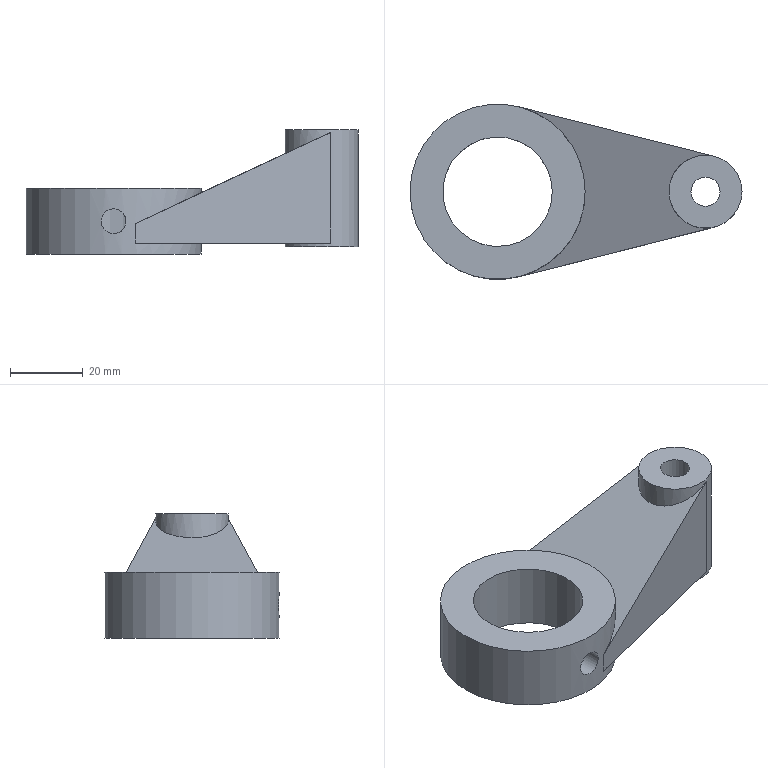Part | NX | features EXTRUDE 6, DATUM_CSYS 5, SKETCH 4, REPLACE_FACE 3, BLEND 2, DATUM_PLANE 1, HOLE PACKAGE 1, SIMPLE HOLE 1, SYMBOLIC_THREAD 1, UNITE 1 | 1 solid | 31 faces | box 91 x 48 x 34 mm | volume 35524 mm3 | plane 13 | cylinder 12 | sphere 4 | spline 2 | commonest cylinder face diameters 4 x6 6.8 x1 8 x1 14.5 x1 20 x1 30 x1
STEP:
#1=CARTESIAN_POINT('',(-3.4,-23.758,9.));
#2=VERTEX_POINT('',#1);
#3=CARTESIAN_POINT('',(-2.662,-23.88,6.333));
#4=CARTESIAN_POINT('',(-3.769,-23.697,9.001));
#5=CARTESIAN_POINT('',(-2.663,-23.88,11.665));
#6=CARTESIAN_POINT('',(-0.003138,-24.06,12.767));
#7=CARTESIAN_POINT('',(2.664,-23.88,11.665));
#8=CARTESIAN_POINT('',(3.767,-23.697,9.001));
#9=CARTESIAN_POINT('',(2.667,-23.879,6.339));
#10=CARTESIAN_POINT('',(0.003174,-24.06,5.232));
#11=CARTESIAN_POINT('',(-2.662,-23.88,6.333));
#12=CARTESIAN_POINT('',(-3.769,-23.697,9.001));
#13=CARTESIAN_POINT('',(-2.663,-23.88,11.665));
#14=B_SPLINE_CURVE_WITH_KNOTS('',3,(#3,#4,#5,#6,#7,#8,#9,#10,#11,#12,#13),.UNSPECIFIED.,.T.,.F.,(1,1,1,1,1,1,1,1,1,1,1,1,1,1,1),(-0.007982,-0.005321,-0.002661,0.,0.002661,0.005321,0.007982,0.01064,0.0133,0.01596,0.01862,0.02128,0.02394,0.02661,0.02927),.UNSPECIFIED.);
#15=EDGE_CURVE('',#2,#2,#14,.T.);
#16=ORIENTED_EDGE('',*,*,#15,.T.);
#17=EDGE_LOOP('',(#16));
#18=FACE_BOUND('',#17,.T.);
#19=CARTESIAN_POINT('',(5.895,23.265,3.));
#20=VERTEX_POINT('',#19);
#21=CARTESIAN_POINT('',(21.457,10.751,3.));
#22=VERTEX_POINT('',#21);
#23=CARTESIAN_POINT('',(0.,0.,3.));
#24=DIRECTION('',(0.,0.,-1.));
#25=DIRECTION('',(1.,0.,0.));
#26=AXIS2_PLACEMENT_3D('',#23,#24,#25);
#27=CIRCLE('',#26,24.);
#28=EDGE_CURVE('',#20,#22,#27,.T.);
#29=ORIENTED_EDGE('',*,*,#28,.T.);
#30=CARTESIAN_POINT('',(21.457,10.751,8.699));
#31=VERTEX_POINT('',#30);
#32=CARTESIAN_POINT('',(21.457,10.751,18.));
#33=DIRECTION('',(0.,0.,-1.));
#34=VECTOR('',#33,1000.);
#35=LINE('',#32,#34);
#36=EDGE_CURVE('',#22,#31,#35,.F.);
#37=ORIENTED_EDGE('',*,*,#36,.T.);
#38=CARTESIAN_POINT('',(21.457,-10.751,8.699));
#39=VERTEX_POINT('',#38);
#40=CARTESIAN_POINT('',(0.,0.,-2.14));
#41=DIRECTION('',(-0.4509,0.,0.8926));
#42=DIRECTION('',(-0.8926,0.,-0.4509));
#43=AXIS2_PLACEMENT_3D('',#40,#41,#42);
#44=ELLIPSE('',#43,26.888,24.);
#45=EDGE_CURVE('',#31,#39,#44,.F.);
#46=ORIENTED_EDGE('',*,*,#45,.T.);
#47=CARTESIAN_POINT('',(21.457,-10.751,3.));
#48=VERTEX_POINT('',#47);
#49=CARTESIAN_POINT('',(21.457,-10.751,18.));
#50=DIRECTION('',(0.,0.,-1.));
#51=VECTOR('',#50,1000.);
#52=LINE('',#49,#51);
#53=EDGE_CURVE('',#39,#48,#52,.T.);
#54=ORIENTED_EDGE('',*,*,#53,.T.);
#55=CARTESIAN_POINT('',(5.895,-23.265,3.));
#56=VERTEX_POINT('',#55);
#57=CARTESIAN_POINT('',(0.,0.,3.));
#58=DIRECTION('',(0.,0.,-1.));
#59=DIRECTION('',(1.,0.,0.));
#60=AXIS2_PLACEMENT_3D('',#57,#58,#59);
#61=CIRCLE('',#60,24.);
#62=EDGE_CURVE('',#48,#56,#61,.T.);
#63=ORIENTED_EDGE('',*,*,#62,.T.);
#64=CARTESIAN_POINT('',(5.895,-23.265,8.332));
#65=VERTEX_POINT('',#64);
#66=CARTESIAN_POINT('',(5.895,-23.265,43.));
#67=DIRECTION('',(0.,0.,-1.));
#68=VECTOR('',#67,1000.);
#69=LINE('',#66,#68);
#70=EDGE_CURVE('',#65,#56,#69,.T.);
#71=ORIENTED_EDGE('',*,*,#70,.F.);
#72=CARTESIAN_POINT('',(5.895,23.265,8.332));
#73=VERTEX_POINT('',#72);
#74=CARTESIAN_POINT('',(0.,0.,5.584));
#75=DIRECTION('',(-0.4226,0.,0.9063));
#76=DIRECTION('',(0.9063,0.,0.4226));
#77=AXIS2_PLACEMENT_3D('',#74,#75,#76);
#78=ELLIPSE('',#77,26.481,24.);
#79=EDGE_CURVE('',#73,#65,#78,.F.);
#80=ORIENTED_EDGE('',*,*,#79,.F.);
#81=CARTESIAN_POINT('',(5.895,23.265,43.));
#82=DIRECTION('',(0.,0.,-1.));
#83=VECTOR('',#82,1000.);
#84=LINE('',#81,#83);
#85=EDGE_CURVE('',#73,#20,#84,.T.);
#86=ORIENTED_EDGE('',*,*,#85,.T.);
#87=EDGE_LOOP('',(#29,#37,#46,#54,#63,#71,#80,#86));
#88=FACE_BOUND('',#87,.T.);
#89=CARTESIAN_POINT('',(24.,0.,0.));
#90=VERTEX_POINT('',#89);
#91=CARTESIAN_POINT('',(0.,0.,0.));
#92=DIRECTION('',(0.,0.,1.));
#93=DIRECTION('',(1.,0.,0.));
#94=AXIS2_PLACEMENT_3D('',#91,#92,#93);
#95=CIRCLE('',#94,24.);
#96=EDGE_CURVE('',#90,#90,#95,.T.);
#97=ORIENTED_EDGE('',*,*,#96,.T.);
#98=EDGE_LOOP('',(#97));
#99=FACE_BOUND('',#98,.T.);
#100=CARTESIAN_POINT('',(24.,0.,18.));
#101=VERTEX_POINT('',#100);
#102=CARTESIAN_POINT('',(0.,0.,18.));
#103=DIRECTION('',(0.,0.,1.));
#104=DIRECTION('',(1.,0.,0.));
#105=AXIS2_PLACEMENT_3D('',#102,#103,#104);
#106=CIRCLE('',#105,24.);
#107=EDGE_CURVE('',#101,#101,#106,.T.);
#108=ORIENTED_EDGE('',*,*,#107,.F.);
#109=EDGE_LOOP('',(#108));
#110=FACE_BOUND('',#109,.T.);
#111=CARTESIAN_POINT('',(0.,0.,18.));
#112=DIRECTION('',(0.,0.,-1.));
#113=DIRECTION('',(-1.,0.,0.));
#114=AXIS2_PLACEMENT_3D('',#111,#112,#113);
#115=CYLINDRICAL_SURFACE('',#114,24.);
#116=ADVANCED_FACE('',(#18,#88,#99,#110),#115,.T.);
#117=CARTESIAN_POINT('',(-3.4,-14.61,9.));
#118=VERTEX_POINT('',#117);
#119=CARTESIAN_POINT('',(-2.662,-14.808,6.333));
#120=CARTESIAN_POINT('',(-3.769,-14.511,9.001));
#121=CARTESIAN_POINT('',(-2.663,-14.807,11.665));
#122=CARTESIAN_POINT('',(-0.00369,-15.096,12.768));
#123=CARTESIAN_POINT('',(2.665,-14.807,11.664));
#124=CARTESIAN_POINT('',(3.767,-14.511,9.001));
#125=CARTESIAN_POINT('',(2.667,-14.807,6.338));
#126=CARTESIAN_POINT('',(0.001855,-15.096,5.232));
#127=CARTESIAN_POINT('',(-2.662,-14.808,6.333));
#128=CARTESIAN_POINT('',(-3.769,-14.511,9.001));
#129=CARTESIAN_POINT('',(-2.663,-14.807,11.665));
#130=B_SPLINE_CURVE_WITH_KNOTS('',3,(#119,#120,#121,#122,#123,#124,#125,#126,#127,#128,#129),.UNSPECIFIED.,.T.,.F.,(1,1,1,1,1,1,1,1,1,1,1,1,1,1,1),(-0.007997,-0.005332,-0.002666,0.,0.002666,0.005332,0.007997,0.01066,0.01333,0.01599,0.01866,0.02133,0.02399,0.02666,0.02932),.UNSPECIFIED.);
#131=EDGE_CURVE('',#118,#118,#130,.T.);
#132=ORIENTED_EDGE('',*,*,#131,.F.);
#133=EDGE_LOOP('',(#132));
#134=FACE_BOUND('',#133,.T.);
#135=CARTESIAN_POINT('',(15.,0.,18.));
#136=VERTEX_POINT('',#135);
#137=CARTESIAN_POINT('',(0.,0.,18.));
#138=DIRECTION('',(0.,0.,1.));
#139=DIRECTION('',(1.,0.,0.));
#140=AXIS2_PLACEMENT_3D('',#137,#138,#139);
#141=CIRCLE('',#140,15.);
#142=EDGE_CURVE('',#136,#136,#141,.T.);
#143=ORIENTED_EDGE('',*,*,#142,.T.);
#144=EDGE_LOOP('',(#143));
#145=FACE_BOUND('',#144,.T.);
#146=CARTESIAN_POINT('',(15.,0.,0.));
#147=VERTEX_POINT('',#146);
#148=CARTESIAN_POINT('',(0.,0.,0.));
#149=DIRECTION('',(0.,0.,1.));
#150=DIRECTION('',(1.,0.,0.));
#151=AXIS2_PLACEMENT_3D('',#148,#149,#150);
#152=CIRCLE('',#151,15.);
#153=EDGE_CURVE('',#147,#147,#152,.T.);
#154=ORIENTED_EDGE('',*,*,#153,.F.);
#155=EDGE_LOOP('',(#154));
#156=FACE_BOUND('',#155,.T.);
#157=CARTESIAN_POINT('',(0.,0.,18.));
#158=DIRECTION('',(0.,0.,-1.));
#159=DIRECTION('',(-1.,0.,0.));
#160=AXIS2_PLACEMENT_3D('',#157,#158,#159);
#161=CYLINDRICAL_SURFACE('',#160,15.);
#162=ADVANCED_FACE('',(#134,#145,#156),#161,.F.);
#163=ORIENTED_EDGE('',*,*,#107,.T.);
#164=EDGE_LOOP('',(#163));
#165=FACE_BOUND('',#164,.T.);
#166=ORIENTED_EDGE('',*,*,#142,.F.);
#167=EDGE_LOOP('',(#166));
#168=FACE_BOUND('',#167,.T.);
#169=CARTESIAN_POINT('',(0.,0.,18.));
#170=DIRECTION('',(0.,0.,1.));
#171=DIRECTION('',(1.,0.,0.));
#172=AXIS2_PLACEMENT_3D('',#169,#170,#171);
#173=PLANE('',#172);
#174=ADVANCED_FACE('',(#165,#168),#173,.T.);
#175=ORIENTED_EDGE('',*,*,#96,.F.);
#176=EDGE_LOOP('',(#175));
#177=FACE_BOUND('',#176,.T.);
#178=ORIENTED_EDGE('',*,*,#153,.T.);
#179=EDGE_LOOP('',(#178));
#180=FACE_BOUND('',#179,.T.);
#181=CARTESIAN_POINT('',(0.,0.,0.));
#182=DIRECTION('',(0.,0.,1.));
#183=DIRECTION('',(1.,0.,0.));
#184=AXIS2_PLACEMENT_3D('',#181,#182,#183);
#185=PLANE('',#184);
#186=ADVANCED_FACE('',(#177,#180),#185,.F.);
#187=CARTESIAN_POINT('',(61.,0.,34.));
#188=VERTEX_POINT('',#187);
#189=CARTESIAN_POINT('',(57.,0.,34.));
#190=DIRECTION('',(0.,0.,1.));
#191=DIRECTION('',(1.,0.,0.));
#192=AXIS2_PLACEMENT_3D('',#189,#190,#191);
#193=CIRCLE('',#192,4.);
#194=EDGE_CURVE('',#188,#188,#193,.T.);
#195=ORIENTED_EDGE('',*,*,#194,.T.);
#196=EDGE_LOOP('',(#195));
#197=FACE_BOUND('',#196,.T.);
#198=CARTESIAN_POINT('',(53.,0.,27.));
#199=VERTEX_POINT('',#198);
#200=CARTESIAN_POINT('',(57.,0.,27.));
#201=DIRECTION('',(0.,0.,-1.));
#202=DIRECTION('',(-1.,0.,0.));
#203=AXIS2_PLACEMENT_3D('',#200,#201,#202);
#204=CIRCLE('',#203,4.);
#205=EDGE_CURVE('',#199,#199,#204,.T.);
#206=ORIENTED_EDGE('',*,*,#205,.T.);
#207=EDGE_LOOP('',(#206));
#208=FACE_BOUND('',#207,.T.);
#209=CARTESIAN_POINT('',(57.,0.,34.));
#210=DIRECTION('',(0.,0.,-1.));
#211=DIRECTION('',(-1.,0.,0.));
#212=AXIS2_PLACEMENT_3D('',#209,#210,#211);
#213=CYLINDRICAL_SURFACE('',#212,4.);
#214=ADVANCED_FACE('',(#197,#208),#213,.F.);
#215=CARTESIAN_POINT('',(48.228,4.802,19.531));
#216=VERTEX_POINT('',#215);
#217=CARTESIAN_POINT('',(48.228,4.802,3.));
#218=VERTEX_POINT('',#217);
#219=CARTESIAN_POINT('',(48.228,4.802,34.));
#220=DIRECTION('',(0.,0.,-1.));
#221=VECTOR('',#220,1000.);
#222=LINE('',#219,#221);
#223=EDGE_CURVE('',#216,#218,#222,.T.);
#224=ORIENTED_EDGE('',*,*,#223,.T.);
#225=CARTESIAN_POINT('',(59.456,9.694,3.));
#226=VERTEX_POINT('',#225);
#227=CARTESIAN_POINT('',(57.,0.,3.));
#228=DIRECTION('',(0.,0.,-1.));
#229=DIRECTION('',(1.,0.,0.));
#230=AXIS2_PLACEMENT_3D('',#227,#228,#229);
#231=CIRCLE('',#230,10.);
#232=EDGE_CURVE('',#218,#226,#231,.T.);
#233=ORIENTED_EDGE('',*,*,#232,.T.);
#234=CARTESIAN_POINT('',(59.456,9.694,33.308));
#235=VERTEX_POINT('',#234);
#236=CARTESIAN_POINT('',(59.456,9.694,30.55));
#237=DIRECTION('',(0.,0.,-1.));
#238=VECTOR('',#237,1000.);
#239=LINE('',#236,#238);
#240=EDGE_CURVE('',#226,#235,#239,.F.);
#241=ORIENTED_EDGE('',*,*,#240,.T.);
#242=CARTESIAN_POINT('',(59.456,-9.694,33.308));
#243=VERTEX_POINT('',#242);
#244=CARTESIAN_POINT('',(57.,0.,32.163));
#245=DIRECTION('',(-0.4226,0.,0.9063));
#246=DIRECTION('',(-0.9063,0.,-0.4226));
#247=AXIS2_PLACEMENT_3D('',#244,#245,#246);
#248=ELLIPSE('',#247,11.034,10.);
#249=EDGE_CURVE('',#235,#243,#248,.T.);
#250=ORIENTED_EDGE('',*,*,#249,.T.);
#251=CARTESIAN_POINT('',(59.456,-9.694,3.));
#252=VERTEX_POINT('',#251);
#253=CARTESIAN_POINT('',(59.456,-9.694,30.55));
#254=DIRECTION('',(0.,0.,-1.));
#255=VECTOR('',#254,1000.);
#256=LINE('',#253,#255);
#257=EDGE_CURVE('',#243,#252,#256,.T.);
#258=ORIENTED_EDGE('',*,*,#257,.T.);
#259=CARTESIAN_POINT('',(48.228,-4.802,3.));
#260=VERTEX_POINT('',#259);
#261=CARTESIAN_POINT('',(57.,0.,3.));
#262=DIRECTION('',(0.,0.,-1.));
#263=DIRECTION('',(1.,0.,0.));
#264=AXIS2_PLACEMENT_3D('',#261,#262,#263);
#265=CIRCLE('',#264,10.);
#266=EDGE_CURVE('',#252,#260,#265,.T.);
#267=ORIENTED_EDGE('',*,*,#266,.T.);
#268=CARTESIAN_POINT('',(48.228,-4.802,19.531));
#269=VERTEX_POINT('',#268);
#270=CARTESIAN_POINT('',(48.228,-4.802,34.));
#271=DIRECTION('',(0.,0.,-1.));
#272=VECTOR('',#271,1000.);
#273=LINE('',#270,#272);
#274=EDGE_CURVE('',#260,#269,#273,.F.);
#275=ORIENTED_EDGE('',*,*,#274,.T.);
#276=CARTESIAN_POINT('',(57.,0.,24.439));
#277=DIRECTION('',(-0.4883,0.,0.8727));
#278=DIRECTION('',(-0.8727,0.,-0.4883));
#279=AXIS2_PLACEMENT_3D('',#276,#277,#278);
#280=ELLIPSE('',#279,11.459,10.);
#281=EDGE_CURVE('',#269,#216,#280,.F.);
#282=ORIENTED_EDGE('',*,*,#281,.T.);
#283=EDGE_LOOP('',(#224,#233,#241,#250,#258,#267,#275,#282));
#284=FACE_BOUND('',#283,.T.);
#285=CARTESIAN_POINT('',(67.,0.,2.));
#286=VERTEX_POINT('',#285);
#287=CARTESIAN_POINT('',(57.,0.,2.));
#288=DIRECTION('',(0.,0.,1.));
#289=DIRECTION('',(1.,0.,0.));
#290=AXIS2_PLACEMENT_3D('',#287,#288,#289);
#291=CIRCLE('',#290,10.);
#292=EDGE_CURVE('',#286,#286,#291,.T.);
#293=ORIENTED_EDGE('',*,*,#292,.T.);
#294=EDGE_LOOP('',(#293));
#295=FACE_BOUND('',#294,.T.);
#296=CARTESIAN_POINT('',(67.,0.,34.));
#297=VERTEX_POINT('',#296);
#298=CARTESIAN_POINT('',(57.,0.,34.));
#299=DIRECTION('',(0.,0.,1.));
#300=DIRECTION('',(1.,0.,0.));
#301=AXIS2_PLACEMENT_3D('',#298,#299,#300);
#302=CIRCLE('',#301,10.);
#303=EDGE_CURVE('',#297,#297,#302,.T.);
#304=ORIENTED_EDGE('',*,*,#303,.F.);
#305=EDGE_LOOP('',(#304));
#306=FACE_BOUND('',#305,.T.);
#307=CARTESIAN_POINT('',(57.,0.,34.));
#308=DIRECTION('',(0.,0.,-1.));
#309=DIRECTION('',(-1.,0.,0.));
#310=AXIS2_PLACEMENT_3D('',#307,#308,#309);
#311=CYLINDRICAL_SURFACE('',#310,10.);
#312=ADVANCED_FACE('',(#284,#295,#306),#311,.T.);
#313=ORIENTED_EDGE('',*,*,#303,.T.);
#314=EDGE_LOOP('',(#313));
#315=FACE_BOUND('',#314,.T.);
#316=ORIENTED_EDGE('',*,*,#194,.F.);
#317=EDGE_LOOP('',(#316));
#318=FACE_BOUND('',#317,.T.);
#319=CARTESIAN_POINT('',(57.,0.,34.));
#320=DIRECTION('',(0.,0.,1.));
#321=DIRECTION('',(1.,0.,0.));
#322=AXIS2_PLACEMENT_3D('',#319,#320,#321);
#323=PLANE('',#322);
#324=ADVANCED_FACE('',(#315,#318),#323,.T.);
#325=CARTESIAN_POINT('',(64.25,0.,2.));
#326=VERTEX_POINT('',#325);
#327=CARTESIAN_POINT('',(57.,0.,2.));
#328=DIRECTION('',(0.,0.,-1.));
#329=DIRECTION('',(1.,0.,0.));
#330=AXIS2_PLACEMENT_3D('',#327,#328,#329);
#331=CIRCLE('',#330,7.25);
#332=EDGE_CURVE('',#326,#326,#331,.T.);
#333=ORIENTED_EDGE('',*,*,#332,.F.);
#334=EDGE_LOOP('',(#333));
#335=FACE_BOUND('',#334,.T.);
#336=ORIENTED_EDGE('',*,*,#292,.F.);
#337=EDGE_LOOP('',(#336));
#338=FACE_BOUND('',#337,.T.);
#339=CARTESIAN_POINT('',(57.,0.,2.));
#340=DIRECTION('',(0.,0.,1.));
#341=DIRECTION('',(1.,0.,0.));
#342=AXIS2_PLACEMENT_3D('',#339,#340,#341);
#343=PLANE('',#342);
#344=ADVANCED_FACE('',(#335,#338),#343,.F.);
#345=CARTESIAN_POINT('',(64.25,0.,27.));
#346=VERTEX_POINT('',#345);
#347=CARTESIAN_POINT('',(57.,0.,27.));
#348=DIRECTION('',(0.,0.,-1.));
#349=DIRECTION('',(1.,0.,0.));
#350=AXIS2_PLACEMENT_3D('',#347,#348,#349);
#351=CIRCLE('',#350,7.25);
#352=EDGE_CURVE('',#346,#346,#351,.F.);
#353=ORIENTED_EDGE('',*,*,#352,.T.);
#354=EDGE_LOOP('',(#353));
#355=FACE_BOUND('',#354,.T.);
#356=ORIENTED_EDGE('',*,*,#332,.T.);
#357=EDGE_LOOP('',(#356));
#358=FACE_BOUND('',#357,.T.);
#359=CARTESIAN_POINT('',(57.,0.,27.));
#360=DIRECTION('',(0.,0.,-1.));
#361=DIRECTION('',(-1.,0.,0.));
#362=AXIS2_PLACEMENT_3D('',#359,#360,#361);
#363=CYLINDRICAL_SURFACE('',#362,7.25);
#364=ADVANCED_FACE('',(#355,#358),#363,.F.);
#365=ORIENTED_EDGE('',*,*,#205,.F.);
#366=EDGE_LOOP('',(#365));
#367=FACE_BOUND('',#366,.T.);
#368=ORIENTED_EDGE('',*,*,#352,.F.);
#369=EDGE_LOOP('',(#368));
#370=FACE_BOUND('',#369,.T.);
#371=CARTESIAN_POINT('',(57.,0.,27.));
#372=DIRECTION('',(0.,0.,-1.));
#373=DIRECTION('',(-1.,0.,0.));
#374=AXIS2_PLACEMENT_3D('',#371,#372,#373);
#375=PLANE('',#374);
#376=ADVANCED_FACE('',(#367,#370),#375,.T.);
#377=CARTESIAN_POINT('',(46.965,-7.701,3.));
#378=VERTEX_POINT('',#377);
#379=CARTESIAN_POINT('',(23.736,-13.586,3.));
#380=VERTEX_POINT('',#379);
#381=CARTESIAN_POINT('',(49.833,-6.974,3.));
#382=DIRECTION('',(-0.9694,-0.2456,0.));
#383=VECTOR('',#382,1000.);
#384=LINE('',#381,#383);
#385=EDGE_CURVE('',#378,#380,#384,.T.);
#386=ORIENTED_EDGE('',*,*,#385,.T.);
#387=CARTESIAN_POINT('',(23.736,-13.586,8.699));
#388=VERTEX_POINT('',#387);
#389=CARTESIAN_POINT('',(23.736,-13.586,6.435));
#390=DIRECTION('',(0.,0.,1.));
#391=VECTOR('',#390,1000.);
#392=LINE('',#389,#391);
#393=EDGE_CURVE('',#380,#388,#392,.T.);
#394=ORIENTED_EDGE('',*,*,#393,.T.);
#395=CARTESIAN_POINT('',(46.965,-7.701,19.531));
#396=VERTEX_POINT('',#395);
#397=CARTESIAN_POINT('',(57.885,-4.934,24.623));
#398=DIRECTION('',(-0.8833,-0.2238,-0.4119));
#399=VECTOR('',#398,1000.);
#400=LINE('',#397,#399);
#401=EDGE_CURVE('',#388,#396,#400,.F.);
#402=ORIENTED_EDGE('',*,*,#401,.T.);
#403=CARTESIAN_POINT('',(46.965,-7.701,3.));
#404=DIRECTION('',(0.,0.,1.));
#405=VECTOR('',#404,1000.);
#406=LINE('',#403,#405);
#407=EDGE_CURVE('',#396,#378,#406,.F.);
#408=ORIENTED_EDGE('',*,*,#407,.T.);
#409=EDGE_LOOP('',(#386,#394,#402,#408));
#410=FACE_BOUND('',#409,.T.);
#411=CARTESIAN_POINT('',(49.833,-6.974,43.));
#412=DIRECTION('',(0.2456,-0.9694,0.));
#413=DIRECTION('',(0.9694,0.2456,0.));
#414=AXIS2_PLACEMENT_3D('',#411,#412,#413);
#415=PLANE('',#414);
#416=ADVANCED_FACE('',(#410),#415,.F.);
#417=ORIENTED_EDGE('',*,*,#62,.F.);
#418=CARTESIAN_POINT('',(23.245,-11.647,3.));
#419=DIRECTION('',(0.,0.,-1.));
#420=DIRECTION('',(-1.,0.,0.));
#421=AXIS2_PLACEMENT_3D('',#418,#419,#420);
#422=CIRCLE('',#421,2.);
#423=EDGE_CURVE('',#48,#380,#422,.F.);
#424=ORIENTED_EDGE('',*,*,#423,.T.);
#425=ORIENTED_EDGE('',*,*,#385,.F.);
#426=CARTESIAN_POINT('',(46.474,-5.762,3.));
#427=DIRECTION('',(0.,0.,-1.));
#428=DIRECTION('',(-1.,0.,0.));
#429=AXIS2_PLACEMENT_3D('',#426,#427,#428);
#430=CIRCLE('',#429,2.);
#431=EDGE_CURVE('',#378,#260,#430,.F.);
#432=ORIENTED_EDGE('',*,*,#431,.T.);
#433=ORIENTED_EDGE('',*,*,#266,.F.);
#434=CARTESIAN_POINT('',(5.895,-23.265,3.));
#435=DIRECTION('',(0.9694,0.2456,0.));
#436=VECTOR('',#435,1000.);
#437=LINE('',#434,#436);
#438=EDGE_CURVE('',#56,#252,#437,.T.);
#439=ORIENTED_EDGE('',*,*,#438,.F.);
#440=EDGE_LOOP('',(#417,#424,#425,#432,#433,#439));
#441=FACE_BOUND('',#440,.T.);
#442=CARTESIAN_POINT('',(0.,0.,3.));
#443=DIRECTION('',(0.,0.,-1.));
#444=DIRECTION('',(-1.,0.,0.));
#445=AXIS2_PLACEMENT_3D('',#442,#443,#444);
#446=PLANE('',#445);
#447=ADVANCED_FACE('',(#441),#446,.T.);
#448=CARTESIAN_POINT('',(46.965,7.701,19.531));
#449=VERTEX_POINT('',#448);
#450=CARTESIAN_POINT('',(23.736,13.586,8.699));
#451=VERTEX_POINT('',#450);
#452=CARTESIAN_POINT('',(32.184,11.446,12.639));
#453=DIRECTION('',(0.8833,-0.2238,0.4119));
#454=VECTOR('',#453,1000.);
#455=LINE('',#452,#454);
#456=EDGE_CURVE('',#449,#451,#455,.F.);
#457=ORIENTED_EDGE('',*,*,#456,.T.);
#458=CARTESIAN_POINT('',(23.736,13.586,3.));
#459=VERTEX_POINT('',#458);
#460=CARTESIAN_POINT('',(23.736,13.586,3.));
#461=DIRECTION('',(0.,0.,1.));
#462=VECTOR('',#461,1000.);
#463=LINE('',#460,#462);
#464=EDGE_CURVE('',#451,#459,#463,.F.);
#465=ORIENTED_EDGE('',*,*,#464,.T.);
#466=CARTESIAN_POINT('',(46.965,7.701,3.));
#467=VERTEX_POINT('',#466);
#468=CARTESIAN_POINT('',(18.88,14.817,3.));
#469=DIRECTION('',(0.9694,-0.2456,0.));
#470=VECTOR('',#469,1000.);
#471=LINE('',#468,#470);
#472=EDGE_CURVE('',#459,#467,#471,.T.);
#473=ORIENTED_EDGE('',*,*,#472,.T.);
#474=CARTESIAN_POINT('',(46.965,7.701,23.304));
#475=DIRECTION('',(0.,0.,1.));
#476=VECTOR('',#475,1000.);
#477=LINE('',#474,#476);
#478=EDGE_CURVE('',#467,#449,#477,.T.);
#479=ORIENTED_EDGE('',*,*,#478,.T.);
#480=EDGE_LOOP('',(#457,#465,#473,#479));
#481=FACE_BOUND('',#480,.T.);
#482=CARTESIAN_POINT('',(18.88,14.817,43.));
#483=DIRECTION('',(0.2456,0.9694,0.));
#484=DIRECTION('',(-0.9694,0.2456,0.));
#485=AXIS2_PLACEMENT_3D('',#482,#483,#484);
#486=PLANE('',#485);
#487=ADVANCED_FACE('',(#481),#486,.F.);
#488=ORIENTED_EDGE('',*,*,#28,.F.);
#489=CARTESIAN_POINT('',(59.456,9.694,3.));
#490=DIRECTION('',(-0.9694,0.2456,0.));
#491=VECTOR('',#490,1000.);
#492=LINE('',#489,#491);
#493=EDGE_CURVE('',#226,#20,#492,.T.);
#494=ORIENTED_EDGE('',*,*,#493,.F.);
#495=ORIENTED_EDGE('',*,*,#232,.F.);
#496=CARTESIAN_POINT('',(46.474,5.762,3.));
#497=DIRECTION('',(0.,0.,-1.));
#498=DIRECTION('',(-1.,0.,0.));
#499=AXIS2_PLACEMENT_3D('',#496,#497,#498);
#500=CIRCLE('',#499,2.);
#501=EDGE_CURVE('',#218,#467,#500,.F.);
#502=ORIENTED_EDGE('',*,*,#501,.T.);
#503=ORIENTED_EDGE('',*,*,#472,.F.);
#504=CARTESIAN_POINT('',(23.245,11.647,3.));
#505=DIRECTION('',(0.,0.,-1.));
#506=DIRECTION('',(-1.,0.,0.));
#507=AXIS2_PLACEMENT_3D('',#504,#505,#506);
#508=CIRCLE('',#507,2.);
#509=EDGE_CURVE('',#459,#22,#508,.F.);
#510=ORIENTED_EDGE('',*,*,#509,.T.);
#511=EDGE_LOOP('',(#488,#494,#495,#502,#503,#510));
#512=FACE_BOUND('',#511,.T.);
#513=CARTESIAN_POINT('',(0.,0.,3.));
#514=DIRECTION('',(0.,0.,-1.));
#515=DIRECTION('',(-1.,0.,0.));
#516=AXIS2_PLACEMENT_3D('',#513,#514,#515);
#517=PLANE('',#516);
#518=ADVANCED_FACE('',(#512),#517,.T.);
#519=ORIENTED_EDGE('',*,*,#85,.F.);
#520=CARTESIAN_POINT('',(44.598,13.458,26.38));
#521=DIRECTION('',(-0.8833,0.2238,-0.4119));
#522=VECTOR('',#521,1000.);
#523=LINE('',#520,#522);
#524=EDGE_CURVE('',#235,#73,#523,.T.);
#525=ORIENTED_EDGE('',*,*,#524,.F.);
#526=ORIENTED_EDGE('',*,*,#240,.F.);
#527=ORIENTED_EDGE('',*,*,#493,.T.);
#528=EDGE_LOOP('',(#519,#525,#526,#527));
#529=FACE_BOUND('',#528,.T.);
#530=CARTESIAN_POINT('',(59.456,9.694,-25.));
#531=DIRECTION('',(0.2456,0.9694,0.));
#532=DIRECTION('',(-0.9694,0.2456,0.));
#533=AXIS2_PLACEMENT_3D('',#530,#531,#532);
#534=PLANE('',#533);
#535=ADVANCED_FACE('',(#529),#534,.T.);
#536=CARTESIAN_POINT('',(54.483,-10.954,30.989));
#537=DIRECTION('',(0.8833,0.2238,0.4119));
#538=VECTOR('',#537,1000.);
#539=LINE('',#536,#538);
#540=EDGE_CURVE('',#65,#243,#539,.T.);
#541=ORIENTED_EDGE('',*,*,#540,.F.);
#542=ORIENTED_EDGE('',*,*,#70,.T.);
#543=ORIENTED_EDGE('',*,*,#438,.T.);
#544=ORIENTED_EDGE('',*,*,#257,.F.);
#545=EDGE_LOOP('',(#541,#542,#543,#544));
#546=FACE_BOUND('',#545,.T.);
#547=CARTESIAN_POINT('',(5.895,-23.265,-25.));
#548=DIRECTION('',(0.2456,-0.9694,0.));
#549=DIRECTION('',(0.9694,0.2456,0.));
#550=AXIS2_PLACEMENT_3D('',#547,#548,#549);
#551=PLANE('',#550);
#552=ADVANCED_FACE('',(#546),#551,.T.);
#553=ORIENTED_EDGE('',*,*,#79,.T.);
#554=ORIENTED_EDGE('',*,*,#540,.T.);
#555=ORIENTED_EDGE('',*,*,#249,.F.);
#556=ORIENTED_EDGE('',*,*,#524,.T.);
#557=EDGE_LOOP('',(#553,#554,#555,#556));
#558=FACE_BOUND('',#557,.T.);
#559=CARTESIAN_POINT('',(47.,25.,27.5));
#560=DIRECTION('',(-0.4226,0.,0.9063));
#561=DIRECTION('',(0.9063,0.,0.4226));
#562=AXIS2_PLACEMENT_3D('',#559,#560,#561);
#563=PLANE('',#562);
#564=ADVANCED_FACE('',(#558),#563,.T.);
#565=CARTESIAN_POINT('',(45.629,-5.762,21.344));
#566=VERTEX_POINT('',#565);
#567=CARTESIAN_POINT('',(22.4,-11.647,10.512));
#568=VERTEX_POINT('',#567);
#569=CARTESIAN_POINT('',(19.614,-12.353,9.213));
#570=DIRECTION('',(-0.8833,-0.2238,-0.4119));
#571=VECTOR('',#570,1000.);
#572=LINE('',#569,#571);
#573=EDGE_CURVE('',#566,#568,#572,.T.);
#574=ORIENTED_EDGE('',*,*,#573,.T.);
#575=CARTESIAN_POINT('',(22.4,11.647,10.512));
#576=VERTEX_POINT('',#575);
#577=CARTESIAN_POINT('',(-0.8452,0.,-0.3275));
#578=DIRECTION('',(0.4226,0.,-0.9063));
#579=DIRECTION('',(-0.9063,0.,-0.4226));
#580=AXIS2_PLACEMENT_3D('',#577,#578,#579);
#581=ELLIPSE('',#580,28.688,26.);
#582=EDGE_CURVE('',#568,#576,#581,.F.);
#583=ORIENTED_EDGE('',*,*,#582,.T.);
#584=CARTESIAN_POINT('',(45.629,5.762,21.344));
#585=VERTEX_POINT('',#584);
#586=CARTESIAN_POINT('',(9.729,14.858,4.603));
#587=DIRECTION('',(0.8833,-0.2238,0.4119));
#588=VECTOR('',#587,1000.);
#589=LINE('',#586,#588);
#590=EDGE_CURVE('',#576,#585,#589,.T.);
#591=ORIENTED_EDGE('',*,*,#590,.T.);
#592=CARTESIAN_POINT('',(56.155,0.,26.252));
#593=DIRECTION('',(0.4226,0.,-0.9063));
#594=DIRECTION('',(-0.9063,0.,-0.4226));
#595=AXIS2_PLACEMENT_3D('',#592,#593,#594);
#596=ELLIPSE('',#595,13.241,12.);
#597=EDGE_CURVE('',#585,#566,#596,.F.);
#598=ORIENTED_EDGE('',*,*,#597,.T.);
#599=EDGE_LOOP('',(#574,#583,#591,#598));
#600=FACE_BOUND('',#599,.T.);
#601=CARTESIAN_POINT('',(11.84,25.,5.588));
#602=DIRECTION('',(0.4226,0.,-0.9063));
#603=DIRECTION('',(-0.9063,0.,-0.4226));
#604=AXIS2_PLACEMENT_3D('',#601,#602,#603);
#605=PLANE('',#604);
#606=ADVANCED_FACE('',(#600),#605,.T.);
#607=ORIENTED_EDGE('',*,*,#401,.F.);
#608=CARTESIAN_POINT('',(23.245,-11.647,8.699));
#609=DIRECTION('',(-0.8833,-0.2238,-0.4119));
#610=DIRECTION('',(-0.4226,0.,0.9063));
#611=AXIS2_PLACEMENT_3D('',#608,#609,#610);
#612=CIRCLE('',#611,2.);
#613=EDGE_CURVE('',#388,#568,#612,.T.);
#614=ORIENTED_EDGE('',*,*,#613,.T.);
#615=ORIENTED_EDGE('',*,*,#573,.F.);
#616=CARTESIAN_POINT('',(46.474,-5.762,19.531));
#617=DIRECTION('',(-0.8833,-0.2238,-0.4119));
#618=DIRECTION('',(-0.4226,0.,0.9063));
#619=AXIS2_PLACEMENT_3D('',#616,#617,#618);
#620=CIRCLE('',#619,2.);
#621=EDGE_CURVE('',#396,#566,#620,.T.);
#622=ORIENTED_EDGE('',*,*,#621,.F.);
#623=EDGE_LOOP('',(#607,#614,#615,#622));
#624=FACE_BOUND('',#623,.T.);
#625=CARTESIAN_POINT('',(20.459,-12.353,7.4));
#626=DIRECTION('',(-0.8833,-0.2238,-0.4119));
#627=DIRECTION('',(-0.4226,0.,0.9063));
#628=AXIS2_PLACEMENT_3D('',#625,#626,#627);
#629=CYLINDRICAL_SURFACE('',#628,2.);
#630=ADVANCED_FACE('',(#624),#629,.F.);
#631=ORIENTED_EDGE('',*,*,#431,.F.);
#632=ORIENTED_EDGE('',*,*,#407,.F.);
#633=CARTESIAN_POINT('',(46.474,-5.762,19.531));
#634=DIRECTION('',(0.,0.,-1.));
#635=DIRECTION('',(0.,1.,0.));
#636=AXIS2_PLACEMENT_3D('',#633,#634,#635);
#637=CIRCLE('',#636,2.);
#638=EDGE_CURVE('',#269,#396,#637,.T.);
#639=ORIENTED_EDGE('',*,*,#638,.F.);
#640=ORIENTED_EDGE('',*,*,#274,.F.);
#641=EDGE_LOOP('',(#631,#632,#639,#640));
#642=FACE_BOUND('',#641,.T.);
#643=CARTESIAN_POINT('',(46.474,-5.762,34.));
#644=DIRECTION('',(0.,0.,-1.));
#645=DIRECTION('',(-1.,0.,0.));
#646=AXIS2_PLACEMENT_3D('',#643,#644,#645);
#647=CYLINDRICAL_SURFACE('',#646,2.);
#648=ADVANCED_FACE('',(#642),#647,.F.);
#649=ORIENTED_EDGE('',*,*,#638,.T.);
#650=ORIENTED_EDGE('',*,*,#621,.T.);
#651=CARTESIAN_POINT('',(46.474,-5.762,19.531));
#652=DIRECTION('',(-0.4686,0.856,-0.2185));
#653=DIRECTION('',(-0.8772,-0.4802,0.));
#654=AXIS2_PLACEMENT_3D('',#651,#652,#653);
#655=CIRCLE('',#654,2.);
#656=EDGE_CURVE('',#269,#566,#655,.F.);
#657=ORIENTED_EDGE('',*,*,#656,.F.);
#658=EDGE_LOOP('',(#649,#650,#657));
#659=FACE_BOUND('',#658,.T.);
#660=CARTESIAN_POINT('',(46.474,-5.762,19.531));
#661=DIRECTION('',(0.,0.,1.));
#662=DIRECTION('',(1.,0.,0.));
#663=AXIS2_PLACEMENT_3D('',#660,#661,#662);
#664=SPHERICAL_SURFACE('',#663,2.);
#665=ADVANCED_FACE('',(#659),#664,.F.);
#666=ORIENTED_EDGE('',*,*,#656,.T.);
#667=ORIENTED_EDGE('',*,*,#597,.F.);
#668=CARTESIAN_POINT('',(46.474,5.762,19.531));
#669=DIRECTION('',(-0.4686,-0.856,-0.2185));
#670=DIRECTION('',(0.8772,-0.4802,0.));
#671=AXIS2_PLACEMENT_3D('',#668,#669,#670);
#672=CIRCLE('',#671,2.);
#673=EDGE_CURVE('',#216,#585,#672,.T.);
#674=ORIENTED_EDGE('',*,*,#673,.F.);
#675=ORIENTED_EDGE('',*,*,#281,.F.);
#676=EDGE_LOOP('',(#666,#667,#674,#675));
#677=FACE_BOUND('',#676,.T.);
#678=CARTESIAN_POINT('',(48.228,-4.802,19.531));
#679=CARTESIAN_POINT('',(47.919,-4.236,22.411));
#680=CARTESIAN_POINT('',(45.629,-5.762,21.344));
#681=CARTESIAN_POINT('',(47.427,-3.337,19.082));
#682=CARTESIAN_POINT('',(47.272,-2.824,22.11));
#683=CARTESIAN_POINT('',(44.667,-4.005,20.895));
#684=CARTESIAN_POINT('',(46.573,0.,18.605));
#685=CARTESIAN_POINT('',(46.72,0.,21.852));
#686=CARTESIAN_POINT('',(43.643,0.,20.418));
#687=CARTESIAN_POINT('',(47.427,3.337,19.082));
#688=CARTESIAN_POINT('',(47.272,2.824,22.11));
#689=CARTESIAN_POINT('',(44.667,4.005,20.895));
#690=CARTESIAN_POINT('',(48.228,4.802,19.531));
#691=CARTESIAN_POINT('',(47.919,4.236,22.411));
#692=CARTESIAN_POINT('',(45.629,5.762,21.344));
#693=(BOUNDED_SURFACE()B_SPLINE_SURFACE(3,2,((#678,#679,#680),(#681,#682,#683),(#684,#685,#686),(#687,#688,#689),(#690,#691,#692)),.UNSPECIFIED.,.F.,.F.,.F.)B_SPLINE_SURFACE_WITH_KNOTS((4,1,4),(3,3),(5.782,6.283,6.784),(0.,1.),.UNSPECIFIED.)GEOMETRIC_REPRESENTATION_ITEM()RATIONAL_B_SPLINE_SURFACE(((1.,0.5609,1.),(1.,0.5458,1.),(1.,0.5288,1.),(1.,0.5458,1.),(1.,0.5609,1.)))REPRESENTATION_ITEM('')SURFACE());
#694=ADVANCED_FACE('',(#677),#693,.F.);
#695=ORIENTED_EDGE('',*,*,#501,.F.);
#696=ORIENTED_EDGE('',*,*,#223,.F.);
#697=CARTESIAN_POINT('',(46.474,5.762,19.531));
#698=DIRECTION('',(0.,0.,-1.));
#699=DIRECTION('',(-1.,0.,0.));
#700=AXIS2_PLACEMENT_3D('',#697,#698,#699);
#701=CIRCLE('',#700,2.);
#702=EDGE_CURVE('',#449,#216,#701,.T.);
#703=ORIENTED_EDGE('',*,*,#702,.F.);
#704=ORIENTED_EDGE('',*,*,#478,.F.);
#705=EDGE_LOOP('',(#695,#696,#703,#704));
#706=FACE_BOUND('',#705,.T.);
#707=CARTESIAN_POINT('',(46.474,5.762,34.));
#708=DIRECTION('',(0.,0.,-1.));
#709=DIRECTION('',(-1.,0.,0.));
#710=AXIS2_PLACEMENT_3D('',#707,#708,#709);
#711=CYLINDRICAL_SURFACE('',#710,2.);
#712=ADVANCED_FACE('',(#706),#711,.F.);
#713=ORIENTED_EDGE('',*,*,#702,.T.);
#714=ORIENTED_EDGE('',*,*,#673,.T.);
#715=CARTESIAN_POINT('',(46.474,5.762,19.531));
#716=DIRECTION('',(-0.8833,0.2238,-0.4119));
#717=DIRECTION('',(-0.4226,0.,0.9063));
#718=AXIS2_PLACEMENT_3D('',#715,#716,#717);
#719=CIRCLE('',#718,2.);
#720=EDGE_CURVE('',#449,#585,#719,.F.);
#721=ORIENTED_EDGE('',*,*,#720,.F.);
#722=EDGE_LOOP('',(#713,#714,#721));
#723=FACE_BOUND('',#722,.T.);
#724=CARTESIAN_POINT('',(46.474,5.762,19.531));
#725=DIRECTION('',(0.,0.,1.));
#726=DIRECTION('',(1.,0.,0.));
#727=AXIS2_PLACEMENT_3D('',#724,#725,#726);
#728=SPHERICAL_SURFACE('',#727,2.);
#729=ADVANCED_FACE('',(#723),#728,.F.);
#730=ORIENTED_EDGE('',*,*,#590,.F.);
#731=CARTESIAN_POINT('',(23.245,11.647,8.699));
#732=DIRECTION('',(0.8833,-0.2238,0.4119));
#733=DIRECTION('',(0.4226,0.,-0.9063));
#734=AXIS2_PLACEMENT_3D('',#731,#732,#733);
#735=CIRCLE('',#734,2.);
#736=EDGE_CURVE('',#576,#451,#735,.F.);
#737=ORIENTED_EDGE('',*,*,#736,.T.);
#738=ORIENTED_EDGE('',*,*,#456,.F.);
#739=ORIENTED_EDGE('',*,*,#720,.T.);
#740=EDGE_LOOP('',(#730,#737,#738,#739));
#741=FACE_BOUND('',#740,.T.);
#742=CARTESIAN_POINT('',(10.574,14.858,2.791));
#743=DIRECTION('',(0.8833,-0.2238,0.4119));
#744=DIRECTION('',(0.4226,0.,-0.9063));
#745=AXIS2_PLACEMENT_3D('',#742,#743,#744);
#746=CYLINDRICAL_SURFACE('',#745,2.);
#747=ADVANCED_FACE('',(#741),#746,.F.);
#748=CARTESIAN_POINT('',(23.245,-11.647,8.699));
#749=DIRECTION('',(0.,0.,-1.));
#750=DIRECTION('',(-1.,0.,0.));
#751=AXIS2_PLACEMENT_3D('',#748,#749,#750);
#752=CIRCLE('',#751,2.);
#753=EDGE_CURVE('',#388,#39,#752,.T.);
#754=ORIENTED_EDGE('',*,*,#753,.F.);
#755=ORIENTED_EDGE('',*,*,#393,.F.);
#756=ORIENTED_EDGE('',*,*,#423,.F.);
#757=ORIENTED_EDGE('',*,*,#53,.F.);
#758=EDGE_LOOP('',(#754,#755,#756,#757));
#759=FACE_BOUND('',#758,.T.);
#760=CARTESIAN_POINT('',(23.245,-11.647,18.));
#761=DIRECTION('',(0.,0.,-1.));
#762=DIRECTION('',(-1.,0.,0.));
#763=AXIS2_PLACEMENT_3D('',#760,#761,#762);
#764=CYLINDRICAL_SURFACE('',#763,2.);
#765=ADVANCED_FACE('',(#759),#764,.F.);
#766=ORIENTED_EDGE('',*,*,#613,.F.);
#767=ORIENTED_EDGE('',*,*,#753,.T.);
#768=CARTESIAN_POINT('',(23.245,-11.647,8.699));
#769=DIRECTION('',(-0.4385,-0.8752,-0.2045));
#770=DIRECTION('',(0.894,-0.448,0.));
#771=AXIS2_PLACEMENT_3D('',#768,#769,#770);
#772=CIRCLE('',#771,2.);
#773=EDGE_CURVE('',#568,#39,#772,.T.);
#774=ORIENTED_EDGE('',*,*,#773,.F.);
#775=EDGE_LOOP('',(#766,#767,#774));
#776=FACE_BOUND('',#775,.T.);
#777=CARTESIAN_POINT('',(23.245,-11.647,8.699));
#778=DIRECTION('',(-0.894,0.448,0.));
#779=DIRECTION('',(-0.448,-0.894,0.));
#780=AXIS2_PLACEMENT_3D('',#777,#778,#779);
#781=SPHERICAL_SURFACE('',#780,2.);
#782=ADVANCED_FACE('',(#776),#781,.F.);
#783=CARTESIAN_POINT('',(23.245,11.647,8.699));
#784=DIRECTION('',(0.4385,-0.8752,0.2045));
#785=DIRECTION('',(0.894,0.448,0.));
#786=AXIS2_PLACEMENT_3D('',#783,#784,#785);
#787=CIRCLE('',#786,2.);
#788=EDGE_CURVE('',#576,#31,#787,.T.);
#789=ORIENTED_EDGE('',*,*,#788,.F.);
#790=ORIENTED_EDGE('',*,*,#582,.F.);
#791=ORIENTED_EDGE('',*,*,#773,.T.);
#792=ORIENTED_EDGE('',*,*,#45,.F.);
#793=EDGE_LOOP('',(#789,#790,#791,#792));
#794=FACE_BOUND('',#793,.T.);
#795=CARTESIAN_POINT('',(21.457,10.751,8.699));
#796=CARTESIAN_POINT('',(21.334,10.997,10.015));
#797=CARTESIAN_POINT('',(22.4,11.647,10.512));
#798=CARTESIAN_POINT('',(23.122,7.429,9.54));
#799=CARTESIAN_POINT('',(23.059,7.648,10.819));
#800=CARTESIAN_POINT('',(24.203,8.048,11.353));
#801=CARTESIAN_POINT('',(24.878,0.,10.428));
#802=CARTESIAN_POINT('',(24.931,0.,11.692));
#803=CARTESIAN_POINT('',(26.106,0.,12.24));
#804=CARTESIAN_POINT('',(23.122,-7.429,9.54));
#805=CARTESIAN_POINT('',(23.059,-7.648,10.819));
#806=CARTESIAN_POINT('',(24.203,-8.048,11.353));
#807=CARTESIAN_POINT('',(21.457,-10.751,8.699));
#808=CARTESIAN_POINT('',(21.334,-10.997,10.015));
#809=CARTESIAN_POINT('',(22.4,-11.647,10.512));
#810=(BOUNDED_SURFACE()B_SPLINE_SURFACE(3,2,((#795,#796,#797),(#798,#799,#800),(#801,#802,#803),(#804,#805,#806),(#807,#808,#809)),.UNSPECIFIED.,.F.,.F.,.F.)B_SPLINE_SURFACE_WITH_KNOTS((4,1,4),(3,3),(2.677,3.142,3.606),(0.,1.),.UNSPECIFIED.)GEOMETRIC_REPRESENTATION_ITEM()RATIONAL_B_SPLINE_SURFACE(((1.,0.83,1.),(1.,0.8388,1.),(1.,0.8479,1.),(1.,0.8388,1.),(1.,0.83,1.)))REPRESENTATION_ITEM('')SURFACE());
#811=ADVANCED_FACE('',(#794),#810,.F.);
#812=ORIENTED_EDGE('',*,*,#736,.F.);
#813=ORIENTED_EDGE('',*,*,#788,.T.);
#814=CARTESIAN_POINT('',(23.245,11.647,8.699));
#815=DIRECTION('',(0.,0.,1.));
#816=DIRECTION('',(0.,-1.,0.));
#817=AXIS2_PLACEMENT_3D('',#814,#815,#816);
#818=CIRCLE('',#817,2.);
#819=EDGE_CURVE('',#451,#31,#818,.T.);
#820=ORIENTED_EDGE('',*,*,#819,.F.);
#821=EDGE_LOOP('',(#812,#813,#820));
#822=FACE_BOUND('',#821,.T.);
#823=CARTESIAN_POINT('',(23.245,11.647,8.699));
#824=DIRECTION('',(-0.894,-0.448,0.));
#825=DIRECTION('',(0.448,-0.894,0.));
#826=AXIS2_PLACEMENT_3D('',#823,#824,#825);
#827=SPHERICAL_SURFACE('',#826,2.);
#828=ADVANCED_FACE('',(#822),#827,.F.);
#829=ORIENTED_EDGE('',*,*,#819,.T.);
#830=ORIENTED_EDGE('',*,*,#36,.F.);
#831=ORIENTED_EDGE('',*,*,#509,.F.);
#832=ORIENTED_EDGE('',*,*,#464,.F.);
#833=EDGE_LOOP('',(#829,#830,#831,#832));
#834=FACE_BOUND('',#833,.T.);
#835=CARTESIAN_POINT('',(23.245,11.647,18.));
#836=DIRECTION('',(0.,0.,-1.));
#837=DIRECTION('',(-1.,0.,0.));
#838=AXIS2_PLACEMENT_3D('',#835,#836,#837);
#839=CYLINDRICAL_SURFACE('',#838,2.);
#840=ADVANCED_FACE('',(#834),#839,.F.);
#841=ORIENTED_EDGE('',*,*,#131,.T.);
#842=EDGE_LOOP('',(#841));
#843=FACE_BOUND('',#842,.T.);
#844=ORIENTED_EDGE('',*,*,#15,.F.);
#845=EDGE_LOOP('',(#844));
#846=FACE_BOUND('',#845,.T.);
#847=CARTESIAN_POINT('',(0.,-24.,9.));
#848=DIRECTION('',(0.,1.,0.));
#849=DIRECTION('',(-1.,0.,0.));
#850=AXIS2_PLACEMENT_3D('',#847,#848,#849);
#851=CYLINDRICAL_SURFACE('',#850,3.4);
#852=ADVANCED_FACE('',(#843,#846),#851,.F.);
#853=CLOSED_SHELL('',(#116,#162,#174,#186,#214,#312,#324,#344,#364,#376,#416,#447,#487,#518,#535,#552,#564,#606,#630,#648,#665,#694,#712,#729,#747,#765,#782,#811,#828,#840,#852));
#854=MANIFOLD_SOLID_BREP('',#853);
#855=(LENGTH_UNIT()NAMED_UNIT(*)SI_UNIT(.MILLI.,.METRE.));
#856=UNCERTAINTY_MEASURE_WITH_UNIT(LENGTH_MEASURE(0.0508),#855,'','');
#857=(NAMED_UNIT(*)PLANE_ANGLE_UNIT()SI_UNIT($,.RADIAN.));
#858=(NAMED_UNIT(*)SI_UNIT($,.STERADIAN.)SOLID_ANGLE_UNIT());
#859=(GEOMETRIC_REPRESENTATION_CONTEXT(3)GLOBAL_UNCERTAINTY_ASSIGNED_CONTEXT((#856))GLOBAL_UNIT_ASSIGNED_CONTEXT((#855,#857,#858))REPRESENTATION_CONTEXT('',''));
#860=ADVANCED_BREP_SHAPE_REPRESENTATION('',(#854),#859);